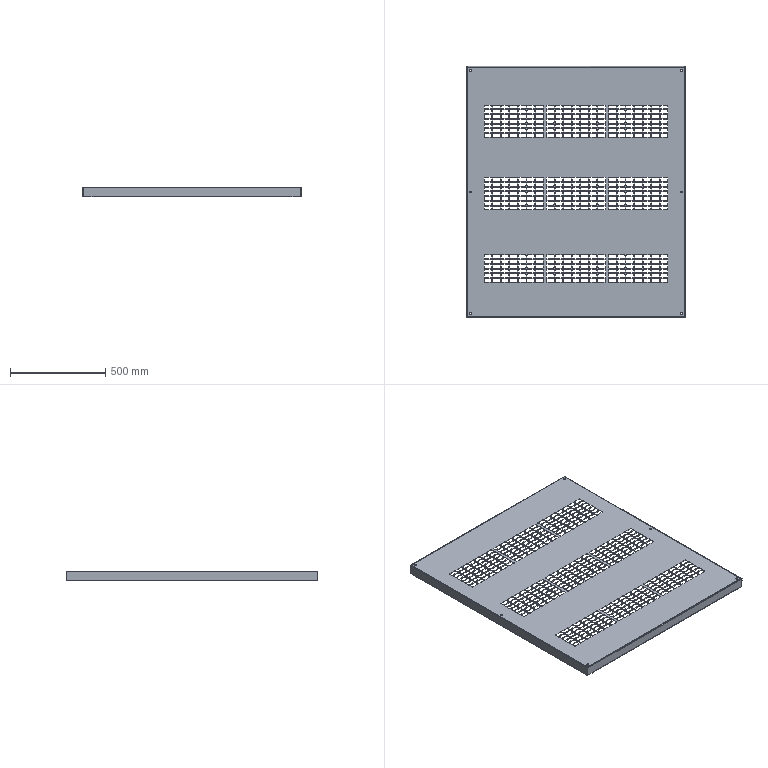Part | STEP file | SYL_0392D6J1SYL0380DJ10-1206392 | 1 solid | 3482 faces | volume 2976644 mm3 | plane 1766 | cylinder 1708 | spline 8 | commonest cylinder face diameters 5 x1680 4 x8 8 x8 10.5 x8 10 x4